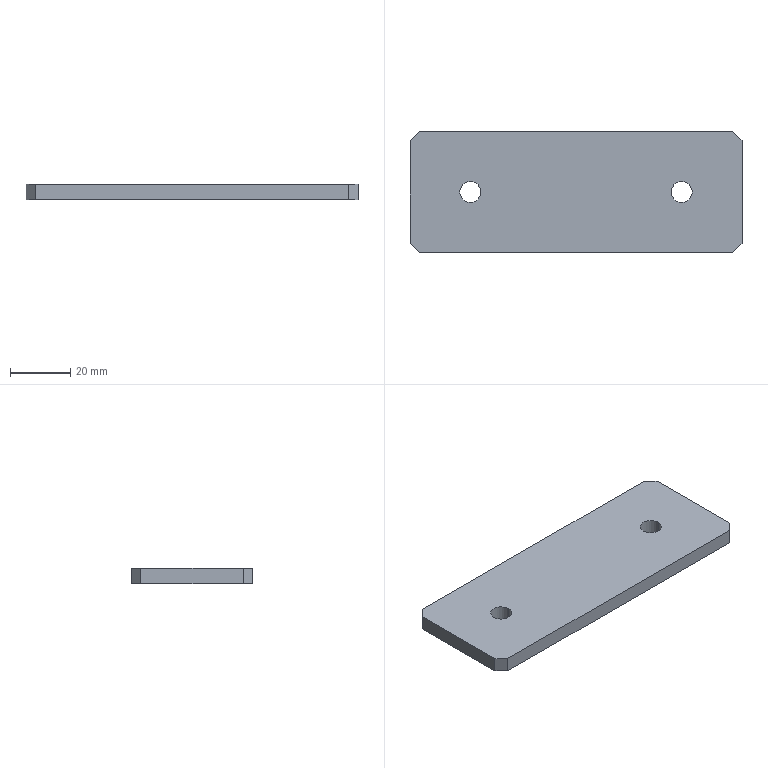Part | SolidWorks | features Chamfer 1, Extrusion 1 | 1 solid | 14 faces | box 110 x 40 x 5 mm | volume 21525 mm3 | plane 10 | cylinder 4 | commonest cylinder face diameters 7 x4
STEP:
#1=CARTESIAN_POINT('',(31.5,0.,5.));
#2=VERTEX_POINT('',#1);
#3=CARTESIAN_POINT('',(38.5,0.,5.));
#4=VERTEX_POINT('',#3);
#5=CARTESIAN_POINT('',(35.,0.,5.));
#6=DIRECTION('',(0.,0.,1.));
#7=DIRECTION('',(1.,0.,0.));
#8=AXIS2_PLACEMENT_3D('',#5,#6,#7);
#9=CIRCLE('',#8,3.5);
#10=EDGE_CURVE('',#2,#4,#9,.T.);
#11=ORIENTED_EDGE('',*,*,#10,.T.);
#12=CARTESIAN_POINT('',(38.5,0.,0.));
#13=VERTEX_POINT('',#12);
#14=CARTESIAN_POINT('',(38.5,0.,5.));
#15=DIRECTION('',(0.,0.,-1.));
#16=VECTOR('',#15,1000.);
#17=LINE('',#14,#16);
#18=EDGE_CURVE('',#4,#13,#17,.T.);
#19=ORIENTED_EDGE('',*,*,#18,.T.);
#20=CARTESIAN_POINT('',(31.5,0.,0.));
#21=VERTEX_POINT('',#20);
#22=CARTESIAN_POINT('',(35.,0.,0.));
#23=DIRECTION('',(0.,0.,1.));
#24=DIRECTION('',(1.,0.,0.));
#25=AXIS2_PLACEMENT_3D('',#22,#23,#24);
#26=CIRCLE('',#25,3.5);
#27=EDGE_CURVE('',#21,#13,#26,.T.);
#28=ORIENTED_EDGE('',*,*,#27,.F.);
#29=CARTESIAN_POINT('',(31.5,0.,5.));
#30=DIRECTION('',(0.,0.,-1.));
#31=VECTOR('',#30,1000.);
#32=LINE('',#29,#31);
#33=EDGE_CURVE('',#2,#21,#32,.T.);
#34=ORIENTED_EDGE('',*,*,#33,.F.);
#35=EDGE_LOOP('',(#11,#19,#28,#34));
#36=FACE_OUTER_BOUND('',#35,.T.);
#37=CARTESIAN_POINT('',(35.,0.,5.));
#38=DIRECTION('',(0.,0.,-1.));
#39=DIRECTION('',(-1.,0.,0.));
#40=AXIS2_PLACEMENT_3D('',#37,#38,#39);
#41=CYLINDRICAL_SURFACE('',#40,3.5);
#42=ADVANCED_FACE('',(#36),#41,.F.);
#43=CARTESIAN_POINT('',(-38.5,0.,5.));
#44=VERTEX_POINT('',#43);
#45=CARTESIAN_POINT('',(-31.5,0.,5.));
#46=VERTEX_POINT('',#45);
#47=CARTESIAN_POINT('',(-35.,0.,5.));
#48=DIRECTION('',(0.,0.,1.));
#49=DIRECTION('',(1.,0.,0.));
#50=AXIS2_PLACEMENT_3D('',#47,#48,#49);
#51=CIRCLE('',#50,3.5);
#52=EDGE_CURVE('',#44,#46,#51,.T.);
#53=ORIENTED_EDGE('',*,*,#52,.T.);
#54=CARTESIAN_POINT('',(-31.5,0.,0.));
#55=VERTEX_POINT('',#54);
#56=CARTESIAN_POINT('',(-31.5,0.,5.));
#57=DIRECTION('',(0.,0.,-1.));
#58=VECTOR('',#57,1000.);
#59=LINE('',#56,#58);
#60=EDGE_CURVE('',#46,#55,#59,.T.);
#61=ORIENTED_EDGE('',*,*,#60,.T.);
#62=CARTESIAN_POINT('',(-38.5,0.,0.));
#63=VERTEX_POINT('',#62);
#64=CARTESIAN_POINT('',(-35.,0.,0.));
#65=DIRECTION('',(0.,0.,1.));
#66=DIRECTION('',(1.,0.,0.));
#67=AXIS2_PLACEMENT_3D('',#64,#65,#66);
#68=CIRCLE('',#67,3.5);
#69=EDGE_CURVE('',#63,#55,#68,.T.);
#70=ORIENTED_EDGE('',*,*,#69,.F.);
#71=CARTESIAN_POINT('',(-38.5,0.,5.));
#72=DIRECTION('',(0.,0.,-1.));
#73=VECTOR('',#72,1000.);
#74=LINE('',#71,#73);
#75=EDGE_CURVE('',#44,#63,#74,.T.);
#76=ORIENTED_EDGE('',*,*,#75,.F.);
#77=EDGE_LOOP('',(#53,#61,#70,#76));
#78=FACE_OUTER_BOUND('',#77,.T.);
#79=CARTESIAN_POINT('',(-35.,0.,5.));
#80=DIRECTION('',(0.,0.,-1.));
#81=DIRECTION('',(-1.,0.,0.));
#82=AXIS2_PLACEMENT_3D('',#79,#80,#81);
#83=CYLINDRICAL_SURFACE('',#82,3.5);
#84=ADVANCED_FACE('',(#78),#83,.F.);
#85=ORIENTED_EDGE('',*,*,#52,.F.);
#86=CARTESIAN_POINT('',(-35.,0.,5.));
#87=DIRECTION('',(0.,0.,1.));
#88=DIRECTION('',(1.,0.,0.));
#89=AXIS2_PLACEMENT_3D('',#86,#87,#88);
#90=CIRCLE('',#89,3.5);
#91=EDGE_CURVE('',#46,#44,#90,.T.);
#92=ORIENTED_EDGE('',*,*,#91,.F.);
#93=EDGE_LOOP('',(#85,#92));
#94=FACE_BOUND('',#93,.T.);
#95=CARTESIAN_POINT('',(52.,20.,5.));
#96=VERTEX_POINT('',#95);
#97=CARTESIAN_POINT('',(-52.,20.,5.));
#98=VERTEX_POINT('',#97);
#99=CARTESIAN_POINT('',(55.,20.,5.));
#100=DIRECTION('',(-1.,0.,0.));
#101=VECTOR('',#100,1000.);
#102=LINE('',#99,#101);
#103=EDGE_CURVE('',#96,#98,#102,.T.);
#104=ORIENTED_EDGE('',*,*,#103,.T.);
#105=CARTESIAN_POINT('',(-55.,17.,5.));
#106=VERTEX_POINT('',#105);
#107=CARTESIAN_POINT('',(-36.,36.,5.));
#108=DIRECTION('',(-0.7071,-0.7071,0.));
#109=VECTOR('',#108,1000.);
#110=LINE('',#107,#109);
#111=EDGE_CURVE('',#98,#106,#110,.T.);
#112=ORIENTED_EDGE('',*,*,#111,.T.);
#113=CARTESIAN_POINT('',(-55.,-17.,5.));
#114=VERTEX_POINT('',#113);
#115=CARTESIAN_POINT('',(-55.,20.,5.));
#116=DIRECTION('',(0.,-1.,0.));
#117=VECTOR('',#116,1000.);
#118=LINE('',#115,#117);
#119=EDGE_CURVE('',#106,#114,#118,.T.);
#120=ORIENTED_EDGE('',*,*,#119,.T.);
#121=CARTESIAN_POINT('',(-52.,-20.,5.));
#122=VERTEX_POINT('',#121);
#123=CARTESIAN_POINT('',(-36.,-36.,5.));
#124=DIRECTION('',(0.7071,-0.7071,0.));
#125=VECTOR('',#124,1000.);
#126=LINE('',#123,#125);
#127=EDGE_CURVE('',#114,#122,#126,.T.);
#128=ORIENTED_EDGE('',*,*,#127,.T.);
#129=CARTESIAN_POINT('',(52.,-20.,5.));
#130=VERTEX_POINT('',#129);
#131=CARTESIAN_POINT('',(55.,-20.,5.));
#132=DIRECTION('',(-1.,0.,0.));
#133=VECTOR('',#132,1000.);
#134=LINE('',#131,#133);
#135=EDGE_CURVE('',#130,#122,#134,.T.);
#136=ORIENTED_EDGE('',*,*,#135,.F.);
#137=CARTESIAN_POINT('',(55.,-17.,5.));
#138=VERTEX_POINT('',#137);
#139=CARTESIAN_POINT('',(36.,-36.,5.));
#140=DIRECTION('',(0.7071,0.7071,0.));
#141=VECTOR('',#140,1000.);
#142=LINE('',#139,#141);
#143=EDGE_CURVE('',#130,#138,#142,.T.);
#144=ORIENTED_EDGE('',*,*,#143,.T.);
#145=CARTESIAN_POINT('',(55.,17.,5.));
#146=VERTEX_POINT('',#145);
#147=CARTESIAN_POINT('',(55.,20.,5.));
#148=DIRECTION('',(0.,-1.,0.));
#149=VECTOR('',#148,1000.);
#150=LINE('',#147,#149);
#151=EDGE_CURVE('',#146,#138,#150,.T.);
#152=ORIENTED_EDGE('',*,*,#151,.F.);
#153=CARTESIAN_POINT('',(36.,36.,5.));
#154=DIRECTION('',(-0.7071,0.7071,0.));
#155=VECTOR('',#154,1000.);
#156=LINE('',#153,#155);
#157=EDGE_CURVE('',#146,#96,#156,.T.);
#158=ORIENTED_EDGE('',*,*,#157,.T.);
#159=EDGE_LOOP('',(#104,#112,#120,#128,#136,#144,#152,#158));
#160=FACE_OUTER_BOUND('',#159,.T.);
#161=ORIENTED_EDGE('',*,*,#10,.F.);
#162=CARTESIAN_POINT('',(35.,0.,5.));
#163=DIRECTION('',(0.,0.,1.));
#164=DIRECTION('',(1.,0.,0.));
#165=AXIS2_PLACEMENT_3D('',#162,#163,#164);
#166=CIRCLE('',#165,3.5);
#167=EDGE_CURVE('',#4,#2,#166,.T.);
#168=ORIENTED_EDGE('',*,*,#167,.F.);
#169=EDGE_LOOP('',(#161,#168));
#170=FACE_BOUND('',#169,.T.);
#171=CARTESIAN_POINT('',(0.,0.,5.));
#172=DIRECTION('',(0.,0.,1.));
#173=DIRECTION('',(1.,0.,0.));
#174=AXIS2_PLACEMENT_3D('',#171,#172,#173);
#175=PLANE('',#174);
#176=ADVANCED_FACE('',(#94,#160,#170),#175,.T.);
#177=CARTESIAN_POINT('',(-55.,17.,0.));
#178=VERTEX_POINT('',#177);
#179=CARTESIAN_POINT('',(-55.,-17.,0.));
#180=VERTEX_POINT('',#179);
#181=CARTESIAN_POINT('',(-55.,20.,0.));
#182=DIRECTION('',(0.,-1.,0.));
#183=VECTOR('',#182,1000.);
#184=LINE('',#181,#183);
#185=EDGE_CURVE('',#178,#180,#184,.T.);
#186=ORIENTED_EDGE('',*,*,#185,.F.);
#187=CARTESIAN_POINT('',(-52.,20.,0.));
#188=VERTEX_POINT('',#187);
#189=CARTESIAN_POINT('',(-55.,17.,0.));
#190=DIRECTION('',(0.7071,0.7071,0.));
#191=VECTOR('',#190,1000.);
#192=LINE('',#189,#191);
#193=EDGE_CURVE('',#178,#188,#192,.T.);
#194=ORIENTED_EDGE('',*,*,#193,.T.);
#195=CARTESIAN_POINT('',(52.,20.,0.));
#196=VERTEX_POINT('',#195);
#197=CARTESIAN_POINT('',(55.,20.,0.));
#198=DIRECTION('',(-1.,0.,0.));
#199=VECTOR('',#198,1000.);
#200=LINE('',#197,#199);
#201=EDGE_CURVE('',#196,#188,#200,.T.);
#202=ORIENTED_EDGE('',*,*,#201,.F.);
#203=CARTESIAN_POINT('',(55.,17.,0.));
#204=VERTEX_POINT('',#203);
#205=CARTESIAN_POINT('',(52.,20.,0.));
#206=DIRECTION('',(0.7071,-0.7071,0.));
#207=VECTOR('',#206,1000.);
#208=LINE('',#205,#207);
#209=EDGE_CURVE('',#196,#204,#208,.T.);
#210=ORIENTED_EDGE('',*,*,#209,.T.);
#211=CARTESIAN_POINT('',(55.,-17.,0.));
#212=VERTEX_POINT('',#211);
#213=CARTESIAN_POINT('',(55.,20.,0.));
#214=DIRECTION('',(0.,-1.,0.));
#215=VECTOR('',#214,1000.);
#216=LINE('',#213,#215);
#217=EDGE_CURVE('',#204,#212,#216,.T.);
#218=ORIENTED_EDGE('',*,*,#217,.T.);
#219=CARTESIAN_POINT('',(52.,-20.,0.));
#220=VERTEX_POINT('',#219);
#221=CARTESIAN_POINT('',(55.,-17.,0.));
#222=DIRECTION('',(-0.7071,-0.7071,0.));
#223=VECTOR('',#222,1000.);
#224=LINE('',#221,#223);
#225=EDGE_CURVE('',#212,#220,#224,.T.);
#226=ORIENTED_EDGE('',*,*,#225,.T.);
#227=CARTESIAN_POINT('',(-52.,-20.,0.));
#228=VERTEX_POINT('',#227);
#229=CARTESIAN_POINT('',(55.,-20.,0.));
#230=DIRECTION('',(-1.,0.,0.));
#231=VECTOR('',#230,1000.);
#232=LINE('',#229,#231);
#233=EDGE_CURVE('',#220,#228,#232,.T.);
#234=ORIENTED_EDGE('',*,*,#233,.T.);
#235=CARTESIAN_POINT('',(-52.,-20.,0.));
#236=DIRECTION('',(-0.7071,0.7071,0.));
#237=VECTOR('',#236,1000.);
#238=LINE('',#235,#237);
#239=EDGE_CURVE('',#228,#180,#238,.T.);
#240=ORIENTED_EDGE('',*,*,#239,.T.);
#241=EDGE_LOOP('',(#186,#194,#202,#210,#218,#226,#234,#240));
#242=FACE_OUTER_BOUND('',#241,.T.);
#243=ORIENTED_EDGE('',*,*,#69,.T.);
#244=CARTESIAN_POINT('',(-35.,0.,0.));
#245=DIRECTION('',(0.,0.,1.));
#246=DIRECTION('',(1.,0.,0.));
#247=AXIS2_PLACEMENT_3D('',#244,#245,#246);
#248=CIRCLE('',#247,3.5);
#249=EDGE_CURVE('',#55,#63,#248,.T.);
#250=ORIENTED_EDGE('',*,*,#249,.T.);
#251=EDGE_LOOP('',(#243,#250));
#252=FACE_BOUND('',#251,.T.);
#253=ORIENTED_EDGE('',*,*,#27,.T.);
#254=CARTESIAN_POINT('',(35.,0.,0.));
#255=DIRECTION('',(0.,0.,1.));
#256=DIRECTION('',(1.,0.,0.));
#257=AXIS2_PLACEMENT_3D('',#254,#255,#256);
#258=CIRCLE('',#257,3.5);
#259=EDGE_CURVE('',#13,#21,#258,.T.);
#260=ORIENTED_EDGE('',*,*,#259,.T.);
#261=EDGE_LOOP('',(#253,#260));
#262=FACE_BOUND('',#261,.T.);
#263=CARTESIAN_POINT('',(0.,0.,0.));
#264=DIRECTION('',(0.,0.,1.));
#265=DIRECTION('',(1.,0.,0.));
#266=AXIS2_PLACEMENT_3D('',#263,#264,#265);
#267=PLANE('',#266);
#268=ADVANCED_FACE('',(#242,#252,#262),#267,.F.);
#269=ORIENTED_EDGE('',*,*,#135,.T.);
#270=CARTESIAN_POINT('',(-52.,-20.,0.));
#271=DIRECTION('',(0.,0.,-1.));
#272=VECTOR('',#271,1000.);
#273=LINE('',#270,#272);
#274=EDGE_CURVE('',#122,#228,#273,.T.);
#275=ORIENTED_EDGE('',*,*,#274,.T.);
#276=ORIENTED_EDGE('',*,*,#233,.F.);
#277=CARTESIAN_POINT('',(52.,-20.,5.));
#278=DIRECTION('',(0.,0.,1.));
#279=VECTOR('',#278,1000.);
#280=LINE('',#277,#279);
#281=EDGE_CURVE('',#220,#130,#280,.T.);
#282=ORIENTED_EDGE('',*,*,#281,.T.);
#283=EDGE_LOOP('',(#269,#275,#276,#282));
#284=FACE_OUTER_BOUND('',#283,.T.);
#285=CARTESIAN_POINT('',(55.,-20.,5.));
#286=DIRECTION('',(0.,-1.,0.));
#287=DIRECTION('',(1.,0.,0.));
#288=AXIS2_PLACEMENT_3D('',#285,#286,#287);
#289=PLANE('',#288);
#290=ADVANCED_FACE('',(#284),#289,.T.);
#291=ORIENTED_EDGE('',*,*,#151,.T.);
#292=CARTESIAN_POINT('',(55.,-17.,5.));
#293=DIRECTION('',(0.,0.,-1.));
#294=VECTOR('',#293,1000.);
#295=LINE('',#292,#294);
#296=EDGE_CURVE('',#138,#212,#295,.T.);
#297=ORIENTED_EDGE('',*,*,#296,.T.);
#298=ORIENTED_EDGE('',*,*,#217,.F.);
#299=CARTESIAN_POINT('',(55.,17.,5.));
#300=DIRECTION('',(0.,0.,1.));
#301=VECTOR('',#300,1000.);
#302=LINE('',#299,#301);
#303=EDGE_CURVE('',#204,#146,#302,.T.);
#304=ORIENTED_EDGE('',*,*,#303,.T.);
#305=EDGE_LOOP('',(#291,#297,#298,#304));
#306=FACE_OUTER_BOUND('',#305,.T.);
#307=CARTESIAN_POINT('',(55.,20.,5.));
#308=DIRECTION('',(1.,0.,0.));
#309=DIRECTION('',(0.,1.,0.));
#310=AXIS2_PLACEMENT_3D('',#307,#308,#309);
#311=PLANE('',#310);
#312=ADVANCED_FACE('',(#306),#311,.T.);
#313=ORIENTED_EDGE('',*,*,#201,.T.);
#314=CARTESIAN_POINT('',(-52.,20.,5.));
#315=DIRECTION('',(0.,0.,1.));
#316=VECTOR('',#315,1000.);
#317=LINE('',#314,#316);
#318=EDGE_CURVE('',#188,#98,#317,.T.);
#319=ORIENTED_EDGE('',*,*,#318,.T.);
#320=ORIENTED_EDGE('',*,*,#103,.F.);
#321=CARTESIAN_POINT('',(52.,20.,0.));
#322=DIRECTION('',(0.,0.,-1.));
#323=VECTOR('',#322,1000.);
#324=LINE('',#321,#323);
#325=EDGE_CURVE('',#96,#196,#324,.T.);
#326=ORIENTED_EDGE('',*,*,#325,.T.);
#327=EDGE_LOOP('',(#313,#319,#320,#326));
#328=FACE_OUTER_BOUND('',#327,.T.);
#329=CARTESIAN_POINT('',(55.,20.,5.));
#330=DIRECTION('',(0.,-1.,0.));
#331=DIRECTION('',(1.,0.,0.));
#332=AXIS2_PLACEMENT_3D('',#329,#330,#331);
#333=PLANE('',#332);
#334=ADVANCED_FACE('',(#328),#333,.F.);
#335=ORIENTED_EDGE('',*,*,#119,.F.);
#336=CARTESIAN_POINT('',(-55.,17.,5.));
#337=DIRECTION('',(0.,0.,-1.));
#338=VECTOR('',#337,1000.);
#339=LINE('',#336,#338);
#340=EDGE_CURVE('',#106,#178,#339,.T.);
#341=ORIENTED_EDGE('',*,*,#340,.T.);
#342=ORIENTED_EDGE('',*,*,#185,.T.);
#343=CARTESIAN_POINT('',(-55.,-17.,5.));
#344=DIRECTION('',(0.,0.,1.));
#345=VECTOR('',#344,1000.);
#346=LINE('',#343,#345);
#347=EDGE_CURVE('',#180,#114,#346,.T.);
#348=ORIENTED_EDGE('',*,*,#347,.T.);
#349=EDGE_LOOP('',(#335,#341,#342,#348));
#350=FACE_OUTER_BOUND('',#349,.T.);
#351=CARTESIAN_POINT('',(-55.,20.,5.));
#352=DIRECTION('',(1.,0.,0.));
#353=DIRECTION('',(0.,0.,-1.));
#354=AXIS2_PLACEMENT_3D('',#351,#352,#353);
#355=PLANE('',#354);
#356=ADVANCED_FACE('',(#350),#355,.F.);
#357=ORIENTED_EDGE('',*,*,#60,.F.);
#358=ORIENTED_EDGE('',*,*,#91,.T.);
#359=ORIENTED_EDGE('',*,*,#75,.T.);
#360=ORIENTED_EDGE('',*,*,#249,.F.);
#361=EDGE_LOOP('',(#357,#358,#359,#360));
#362=FACE_OUTER_BOUND('',#361,.T.);
#363=CARTESIAN_POINT('',(-35.,0.,5.));
#364=DIRECTION('',(0.,0.,-1.));
#365=DIRECTION('',(-1.,0.,0.));
#366=AXIS2_PLACEMENT_3D('',#363,#364,#365);
#367=CYLINDRICAL_SURFACE('',#366,3.5);
#368=ADVANCED_FACE('',(#362),#367,.F.);
#369=ORIENTED_EDGE('',*,*,#18,.F.);
#370=ORIENTED_EDGE('',*,*,#167,.T.);
#371=ORIENTED_EDGE('',*,*,#33,.T.);
#372=ORIENTED_EDGE('',*,*,#259,.F.);
#373=EDGE_LOOP('',(#369,#370,#371,#372));
#374=FACE_OUTER_BOUND('',#373,.T.);
#375=CARTESIAN_POINT('',(35.,0.,5.));
#376=DIRECTION('',(0.,0.,-1.));
#377=DIRECTION('',(-1.,0.,0.));
#378=AXIS2_PLACEMENT_3D('',#375,#376,#377);
#379=CYLINDRICAL_SURFACE('',#378,3.5);
#380=ADVANCED_FACE('',(#374),#379,.F.);
#381=ORIENTED_EDGE('',*,*,#111,.F.);
#382=ORIENTED_EDGE('',*,*,#318,.F.);
#383=ORIENTED_EDGE('',*,*,#193,.F.);
#384=ORIENTED_EDGE('',*,*,#340,.F.);
#385=EDGE_LOOP('',(#381,#382,#383,#384));
#386=FACE_OUTER_BOUND('',#385,.T.);
#387=CARTESIAN_POINT('',(-55.,17.,5.));
#388=DIRECTION('',(0.7071,-0.7071,0.));
#389=DIRECTION('',(0.,0.,-1.));
#390=AXIS2_PLACEMENT_3D('',#387,#388,#389);
#391=PLANE('',#390);
#392=ADVANCED_FACE('',(#386),#391,.F.);
#393=ORIENTED_EDGE('',*,*,#127,.F.);
#394=ORIENTED_EDGE('',*,*,#347,.F.);
#395=ORIENTED_EDGE('',*,*,#239,.F.);
#396=ORIENTED_EDGE('',*,*,#274,.F.);
#397=EDGE_LOOP('',(#393,#394,#395,#396));
#398=FACE_OUTER_BOUND('',#397,.T.);
#399=CARTESIAN_POINT('',(-52.,-20.,5.));
#400=DIRECTION('',(-0.7071,-0.7071,0.));
#401=DIRECTION('',(0.,0.,1.));
#402=AXIS2_PLACEMENT_3D('',#399,#400,#401);
#403=PLANE('',#402);
#404=ADVANCED_FACE('',(#398),#403,.T.);
#405=ORIENTED_EDGE('',*,*,#143,.F.);
#406=ORIENTED_EDGE('',*,*,#281,.F.);
#407=ORIENTED_EDGE('',*,*,#225,.F.);
#408=ORIENTED_EDGE('',*,*,#296,.F.);
#409=EDGE_LOOP('',(#405,#406,#407,#408));
#410=FACE_OUTER_BOUND('',#409,.T.);
#411=CARTESIAN_POINT('',(55.,-17.,5.));
#412=DIRECTION('',(-0.7071,0.7071,0.));
#413=DIRECTION('',(0.,0.,-1.));
#414=AXIS2_PLACEMENT_3D('',#411,#412,#413);
#415=PLANE('',#414);
#416=ADVANCED_FACE('',(#410),#415,.F.);
#417=ORIENTED_EDGE('',*,*,#157,.F.);
#418=ORIENTED_EDGE('',*,*,#303,.F.);
#419=ORIENTED_EDGE('',*,*,#209,.F.);
#420=ORIENTED_EDGE('',*,*,#325,.F.);
#421=EDGE_LOOP('',(#417,#418,#419,#420));
#422=FACE_OUTER_BOUND('',#421,.T.);
#423=CARTESIAN_POINT('',(52.,20.,5.));
#424=DIRECTION('',(0.7071,0.7071,0.));
#425=DIRECTION('',(0.,0.,1.));
#426=AXIS2_PLACEMENT_3D('',#423,#424,#425);
#427=PLANE('',#426);
#428=ADVANCED_FACE('',(#422),#427,.T.);
#429=CLOSED_SHELL('',(#42,#84,#176,#268,#290,#312,#334,#356,#368,#380,#392,#404,#416,#428));
#430=MANIFOLD_SOLID_BREP('',#429);
#431=CARTESIAN_POINT('',(0.,0.,0.));
#432=DIRECTION('',(0.,0.,1.));
#433=DIRECTION('',(1.,0.,0.));
#434=AXIS2_PLACEMENT_3D('',#431,#432,#433);
#435=(LENGTH_UNIT()NAMED_UNIT(*)SI_UNIT(.MILLI.,.METRE.));
#436=UNCERTAINTY_MEASURE_WITH_UNIT(LENGTH_MEASURE(0.00001),#435,'','');
#437=(NAMED_UNIT(*)PLANE_ANGLE_UNIT()SI_UNIT($,.RADIAN.));
#438=(NAMED_UNIT(*)SI_UNIT($,.STERADIAN.)SOLID_ANGLE_UNIT());
#439=(GEOMETRIC_REPRESENTATION_CONTEXT(3)GLOBAL_UNCERTAINTY_ASSIGNED_CONTEXT((#436))GLOBAL_UNIT_ASSIGNED_CONTEXT((#435,#437,#438))REPRESENTATION_CONTEXT('',''));
#440=ADVANCED_BREP_SHAPE_REPRESENTATION('',(#430,#434),#439);